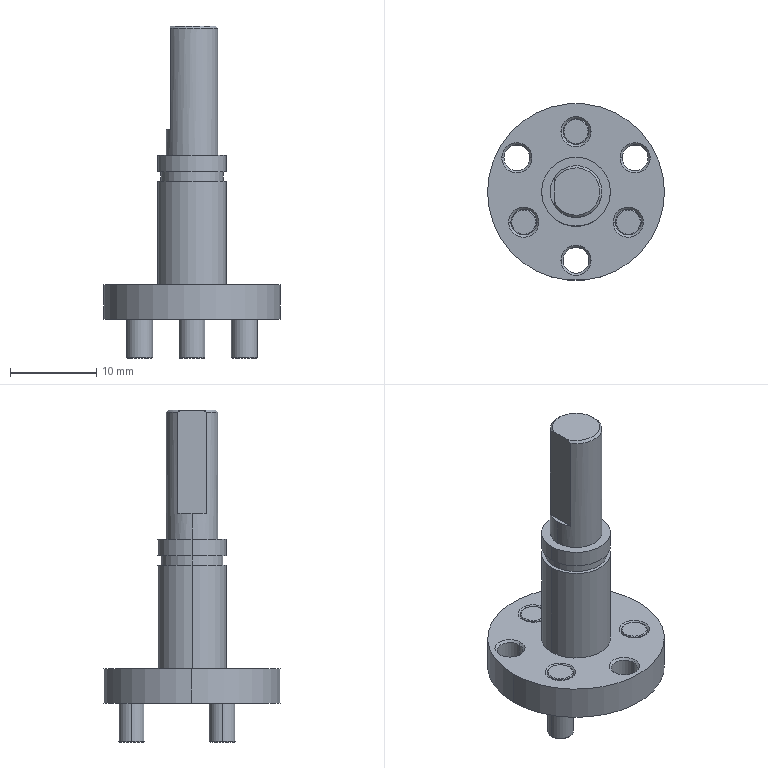Part | SolidWorks | features BaseBody 1 | 1 solid | 88 faces | box 20.5 x 20.5 x 38.5 mm | volume 2479 mm3 | cone 29 | cylinder 28 | plane 19 | torus 12 | commonest cylinder face diameters 3 x18 8 x4 6 x2 7.2 x2 20.5 x2